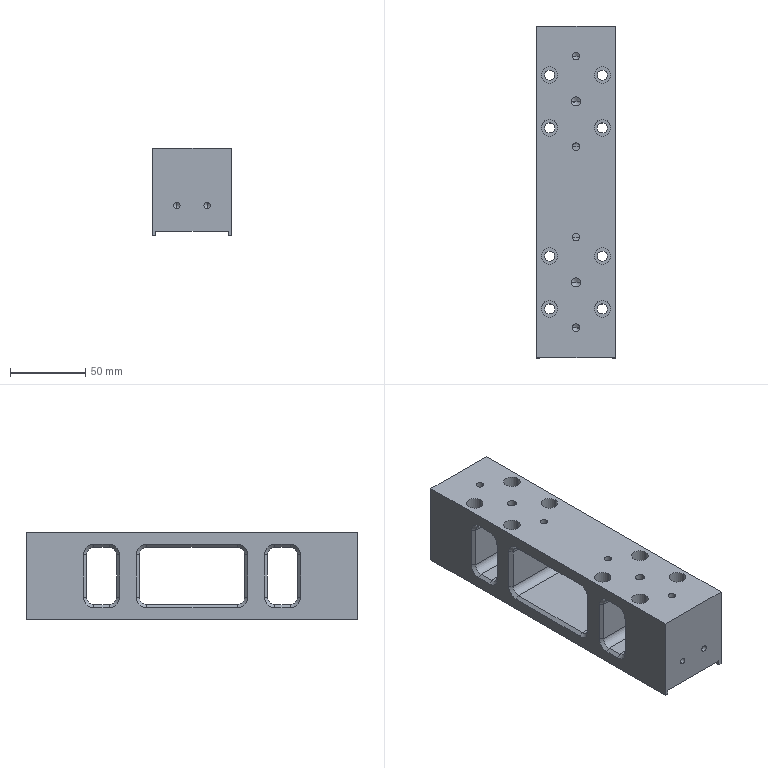Part | SolidWorks | features BaseBody 1 | 1 solid | 158 faces | box 52 x 220 x 58 mm | volume 378968 mm3 | cylinder 64 | plane 54 | cone 40 | commonest cylinder face diameters 6.6 x16 11 x16 10 x12 4.2 x8 5 x8 6 x4